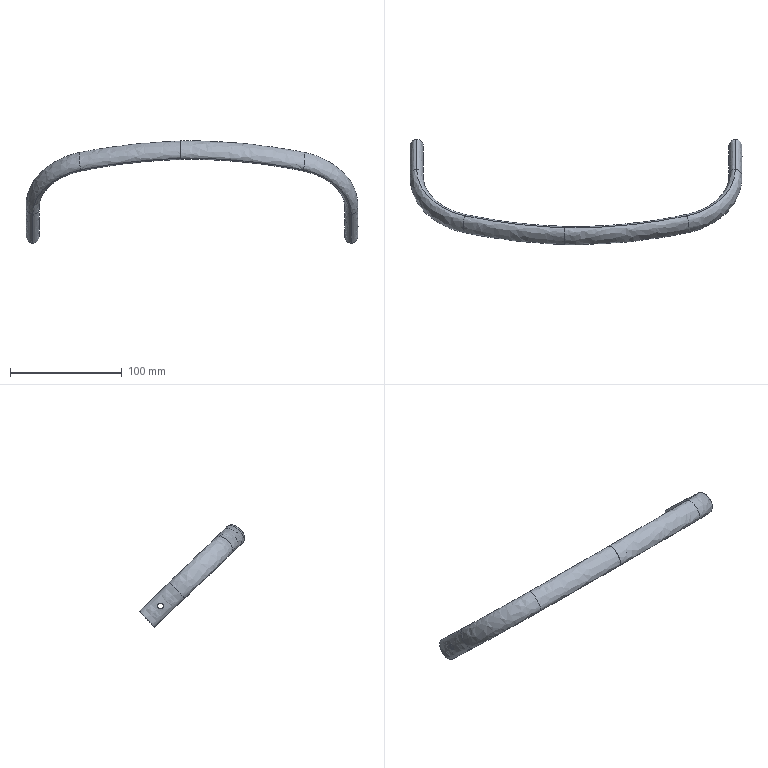Part | SolidWorks | features BaseBody 1 | 1 solid | 38 faces | box 297.02 x 94.548 x 91.608 mm | volume 24402 mm3 | spline 26 | cylinder 8 | plane 4 | commonest cylinder face diameters 5.2 x8